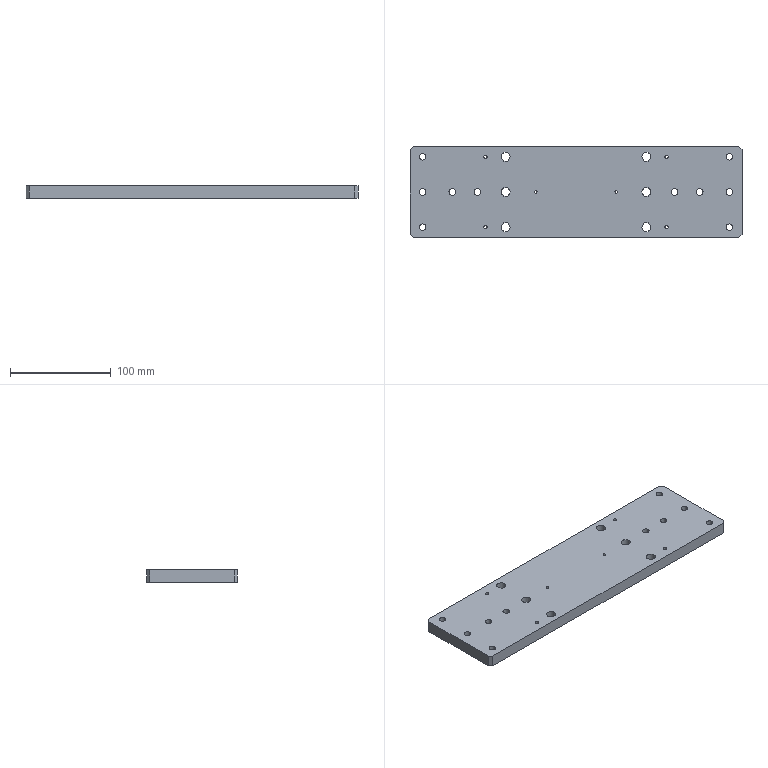Part | 1 solid | 52 faces | box 330 x 90 x 12 mm | volume 343077 mm3 | cylinder 32 | plane 20 | commonest cylinder face diameters 6.6 x10 11 x10 9 x6 3.3 x4 2.5 x2
STEP:
#1=CARTESIAN_POINT('',(147.,35.,0.4));
#2=VERTEX_POINT('',#1);
#3=CARTESIAN_POINT('',(152.5,35.,0.4));
#4=DIRECTION('',(0.,0.,-1.));
#5=DIRECTION('',(-1.,0.,0.));
#6=AXIS2_PLACEMENT_3D('',#3,#4,#5);
#7=CIRCLE('',#6,5.5);
#8=EDGE_CURVE('',#2,#2,#7,.T.);
#9=ORIENTED_EDGE('',*,*,#8,.T.);
#10=EDGE_LOOP('',(#9));
#11=FACE_BOUND('',#10,.T.);
#12=CARTESIAN_POINT('',(149.2,35.,0.4));
#13=VERTEX_POINT('',#12);
#14=CARTESIAN_POINT('',(152.5,35.,0.4));
#15=DIRECTION('',(0.,0.,-1.));
#16=DIRECTION('',(-1.,0.,0.));
#17=AXIS2_PLACEMENT_3D('',#14,#15,#16);
#18=CIRCLE('',#17,3.3);
#19=EDGE_CURVE('',#13,#13,#18,.T.);
#20=ORIENTED_EDGE('',*,*,#19,.F.);
#21=EDGE_LOOP('',(#20));
#22=FACE_BOUND('',#21,.T.);
#23=CARTESIAN_POINT('',(155.8,35.,0.4));
#24=DIRECTION('',(0.,0.,1.));
#25=DIRECTION('',(1.,0.,0.));
#26=AXIS2_PLACEMENT_3D('',#23,#24,#25);
#27=PLANE('',#26);
#28=ADVANCED_FACE('',(#11,#22),#27,.F.);
#29=CARTESIAN_POINT('',(158.,0.,0.4));
#30=VERTEX_POINT('',#29);
#31=CARTESIAN_POINT('',(152.5,0.,0.4));
#32=DIRECTION('',(0.,0.,-1.));
#33=DIRECTION('',(1.,0.,0.));
#34=AXIS2_PLACEMENT_3D('',#31,#32,#33);
#35=CIRCLE('',#34,5.5);
#36=EDGE_CURVE('',#30,#30,#35,.T.);
#37=ORIENTED_EDGE('',*,*,#36,.T.);
#38=EDGE_LOOP('',(#37));
#39=FACE_BOUND('',#38,.T.);
#40=CARTESIAN_POINT('',(155.8,0.,0.4));
#41=VERTEX_POINT('',#40);
#42=CARTESIAN_POINT('',(152.5,0.,0.4));
#43=DIRECTION('',(0.,0.,-1.));
#44=DIRECTION('',(1.,0.,0.));
#45=AXIS2_PLACEMENT_3D('',#42,#43,#44);
#46=CIRCLE('',#45,3.3);
#47=EDGE_CURVE('',#41,#41,#46,.T.);
#48=ORIENTED_EDGE('',*,*,#47,.F.);
#49=EDGE_LOOP('',(#48));
#50=FACE_BOUND('',#49,.T.);
#51=CARTESIAN_POINT('',(155.8,35.,0.4));
#52=DIRECTION('',(0.,0.,1.));
#53=DIRECTION('',(1.,0.,0.));
#54=AXIS2_PLACEMENT_3D('',#51,#52,#53);
#55=PLANE('',#54);
#56=ADVANCED_FACE('',(#39,#50),#55,.F.);
#57=CARTESIAN_POINT('',(128.5,0.,0.4));
#58=VERTEX_POINT('',#57);
#59=CARTESIAN_POINT('',(123.,0.,0.4));
#60=DIRECTION('',(0.,0.,-1.));
#61=DIRECTION('',(1.,0.,0.));
#62=AXIS2_PLACEMENT_3D('',#59,#60,#61);
#63=CIRCLE('',#62,5.5);
#64=EDGE_CURVE('',#58,#58,#63,.T.);
#65=ORIENTED_EDGE('',*,*,#64,.T.);
#66=EDGE_LOOP('',(#65));
#67=FACE_BOUND('',#66,.T.);
#68=CARTESIAN_POINT('',(126.3,0.,0.4));
#69=VERTEX_POINT('',#68);
#70=CARTESIAN_POINT('',(123.,0.,0.4));
#71=DIRECTION('',(0.,0.,-1.));
#72=DIRECTION('',(1.,0.,0.));
#73=AXIS2_PLACEMENT_3D('',#70,#71,#72);
#74=CIRCLE('',#73,3.3);
#75=EDGE_CURVE('',#69,#69,#74,.T.);
#76=ORIENTED_EDGE('',*,*,#75,.F.);
#77=EDGE_LOOP('',(#76));
#78=FACE_BOUND('',#77,.T.);
#79=CARTESIAN_POINT('',(155.8,35.,0.4));
#80=DIRECTION('',(0.,0.,1.));
#81=DIRECTION('',(1.,0.,0.));
#82=AXIS2_PLACEMENT_3D('',#79,#80,#81);
#83=PLANE('',#82);
#84=ADVANCED_FACE('',(#67,#78),#83,.F.);
#85=CARTESIAN_POINT('',(103.5,0.,0.4));
#86=VERTEX_POINT('',#85);
#87=CARTESIAN_POINT('',(98.,0.,0.4));
#88=DIRECTION('',(0.,0.,-1.));
#89=DIRECTION('',(1.,0.,0.));
#90=AXIS2_PLACEMENT_3D('',#87,#88,#89);
#91=CIRCLE('',#90,5.5);
#92=EDGE_CURVE('',#86,#86,#91,.T.);
#93=ORIENTED_EDGE('',*,*,#92,.T.);
#94=EDGE_LOOP('',(#93));
#95=FACE_BOUND('',#94,.T.);
#96=CARTESIAN_POINT('',(101.3,0.,0.4));
#97=VERTEX_POINT('',#96);
#98=CARTESIAN_POINT('',(98.,0.,0.4));
#99=DIRECTION('',(0.,0.,-1.));
#100=DIRECTION('',(1.,0.,0.));
#101=AXIS2_PLACEMENT_3D('',#98,#99,#100);
#102=CIRCLE('',#101,3.3);
#103=EDGE_CURVE('',#97,#97,#102,.T.);
#104=ORIENTED_EDGE('',*,*,#103,.F.);
#105=EDGE_LOOP('',(#104));
#106=FACE_BOUND('',#105,.T.);
#107=CARTESIAN_POINT('',(155.8,35.,0.4));
#108=DIRECTION('',(0.,0.,1.));
#109=DIRECTION('',(1.,0.,0.));
#110=AXIS2_PLACEMENT_3D('',#107,#108,#109);
#111=PLANE('',#110);
#112=ADVANCED_FACE('',(#95,#106),#111,.F.);
#113=CARTESIAN_POINT('',(158.,-35.,0.4));
#114=VERTEX_POINT('',#113);
#115=CARTESIAN_POINT('',(152.5,-35.,0.4));
#116=DIRECTION('',(0.,0.,-1.));
#117=DIRECTION('',(1.,0.,0.));
#118=AXIS2_PLACEMENT_3D('',#115,#116,#117);
#119=CIRCLE('',#118,5.5);
#120=EDGE_CURVE('',#114,#114,#119,.T.);
#121=ORIENTED_EDGE('',*,*,#120,.T.);
#122=EDGE_LOOP('',(#121));
#123=FACE_BOUND('',#122,.T.);
#124=CARTESIAN_POINT('',(155.8,-35.,0.4));
#125=VERTEX_POINT('',#124);
#126=CARTESIAN_POINT('',(152.5,-35.,0.4));
#127=DIRECTION('',(0.,0.,-1.));
#128=DIRECTION('',(1.,0.,0.));
#129=AXIS2_PLACEMENT_3D('',#126,#127,#128);
#130=CIRCLE('',#129,3.3);
#131=EDGE_CURVE('',#125,#125,#130,.T.);
#132=ORIENTED_EDGE('',*,*,#131,.F.);
#133=EDGE_LOOP('',(#132));
#134=FACE_BOUND('',#133,.T.);
#135=CARTESIAN_POINT('',(155.8,35.,0.4));
#136=DIRECTION('',(0.,0.,1.));
#137=DIRECTION('',(1.,0.,0.));
#138=AXIS2_PLACEMENT_3D('',#135,#136,#137);
#139=PLANE('',#138);
#140=ADVANCED_FACE('',(#123,#134),#139,.F.);
#141=CARTESIAN_POINT('',(-147.,-35.,0.4));
#142=VERTEX_POINT('',#141);
#143=CARTESIAN_POINT('',(-152.5,-35.,0.4));
#144=DIRECTION('',(0.,0.,-1.));
#145=DIRECTION('',(1.,0.,0.));
#146=AXIS2_PLACEMENT_3D('',#143,#144,#145);
#147=CIRCLE('',#146,5.5);
#148=EDGE_CURVE('',#142,#142,#147,.T.);
#149=ORIENTED_EDGE('',*,*,#148,.T.);
#150=EDGE_LOOP('',(#149));
#151=FACE_BOUND('',#150,.T.);
#152=CARTESIAN_POINT('',(-149.2,-35.,0.4));
#153=VERTEX_POINT('',#152);
#154=CARTESIAN_POINT('',(-152.5,-35.,0.4));
#155=DIRECTION('',(0.,0.,-1.));
#156=DIRECTION('',(1.,0.,0.));
#157=AXIS2_PLACEMENT_3D('',#154,#155,#156);
#158=CIRCLE('',#157,3.3);
#159=EDGE_CURVE('',#153,#153,#158,.T.);
#160=ORIENTED_EDGE('',*,*,#159,.F.);
#161=EDGE_LOOP('',(#160));
#162=FACE_BOUND('',#161,.T.);
#163=CARTESIAN_POINT('',(155.8,35.,0.4));
#164=DIRECTION('',(0.,0.,1.));
#165=DIRECTION('',(1.,0.,0.));
#166=AXIS2_PLACEMENT_3D('',#163,#164,#165);
#167=PLANE('',#166);
#168=ADVANCED_FACE('',(#151,#162),#167,.F.);
#169=CARTESIAN_POINT('',(-92.5,0.,0.4));
#170=VERTEX_POINT('',#169);
#171=CARTESIAN_POINT('',(-98.,0.,0.4));
#172=DIRECTION('',(0.,0.,-1.));
#173=DIRECTION('',(1.,0.,0.));
#174=AXIS2_PLACEMENT_3D('',#171,#172,#173);
#175=CIRCLE('',#174,5.5);
#176=EDGE_CURVE('',#170,#170,#175,.T.);
#177=ORIENTED_EDGE('',*,*,#176,.T.);
#178=EDGE_LOOP('',(#177));
#179=FACE_BOUND('',#178,.T.);
#180=CARTESIAN_POINT('',(-94.7,0.,0.4));
#181=VERTEX_POINT('',#180);
#182=CARTESIAN_POINT('',(-98.,0.,0.4));
#183=DIRECTION('',(0.,0.,-1.));
#184=DIRECTION('',(1.,0.,0.));
#185=AXIS2_PLACEMENT_3D('',#182,#183,#184);
#186=CIRCLE('',#185,3.3);
#187=EDGE_CURVE('',#181,#181,#186,.T.);
#188=ORIENTED_EDGE('',*,*,#187,.F.);
#189=EDGE_LOOP('',(#188));
#190=FACE_BOUND('',#189,.T.);
#191=CARTESIAN_POINT('',(155.8,35.,0.4));
#192=DIRECTION('',(0.,0.,1.));
#193=DIRECTION('',(1.,0.,0.));
#194=AXIS2_PLACEMENT_3D('',#191,#192,#193);
#195=PLANE('',#194);
#196=ADVANCED_FACE('',(#179,#190),#195,.F.);
#197=CARTESIAN_POINT('',(-117.5,0.,0.4));
#198=VERTEX_POINT('',#197);
#199=CARTESIAN_POINT('',(-123.,0.,0.4));
#200=DIRECTION('',(0.,0.,-1.));
#201=DIRECTION('',(1.,0.,0.));
#202=AXIS2_PLACEMENT_3D('',#199,#200,#201);
#203=CIRCLE('',#202,5.5);
#204=EDGE_CURVE('',#198,#198,#203,.T.);
#205=ORIENTED_EDGE('',*,*,#204,.T.);
#206=EDGE_LOOP('',(#205));
#207=FACE_BOUND('',#206,.T.);
#208=CARTESIAN_POINT('',(-119.7,0.,0.4));
#209=VERTEX_POINT('',#208);
#210=CARTESIAN_POINT('',(-123.,0.,0.4));
#211=DIRECTION('',(0.,0.,-1.));
#212=DIRECTION('',(1.,0.,0.));
#213=AXIS2_PLACEMENT_3D('',#210,#211,#212);
#214=CIRCLE('',#213,3.3);
#215=EDGE_CURVE('',#209,#209,#214,.T.);
#216=ORIENTED_EDGE('',*,*,#215,.F.);
#217=EDGE_LOOP('',(#216));
#218=FACE_BOUND('',#217,.T.);
#219=CARTESIAN_POINT('',(155.8,35.,0.4));
#220=DIRECTION('',(0.,0.,1.));
#221=DIRECTION('',(1.,0.,0.));
#222=AXIS2_PLACEMENT_3D('',#219,#220,#221);
#223=PLANE('',#222);
#224=ADVANCED_FACE('',(#207,#218),#223,.F.);
#225=CARTESIAN_POINT('',(-147.,0.,0.4));
#226=VERTEX_POINT('',#225);
#227=CARTESIAN_POINT('',(-152.5,0.,0.4));
#228=DIRECTION('',(0.,0.,-1.));
#229=DIRECTION('',(1.,0.,0.));
#230=AXIS2_PLACEMENT_3D('',#227,#228,#229);
#231=CIRCLE('',#230,5.5);
#232=EDGE_CURVE('',#226,#226,#231,.T.);
#233=ORIENTED_EDGE('',*,*,#232,.T.);
#234=EDGE_LOOP('',(#233));
#235=FACE_BOUND('',#234,.T.);
#236=CARTESIAN_POINT('',(-149.2,0.,0.4));
#237=VERTEX_POINT('',#236);
#238=CARTESIAN_POINT('',(-152.5,0.,0.4));
#239=DIRECTION('',(0.,0.,-1.));
#240=DIRECTION('',(1.,0.,0.));
#241=AXIS2_PLACEMENT_3D('',#238,#239,#240);
#242=CIRCLE('',#241,3.3);
#243=EDGE_CURVE('',#237,#237,#242,.T.);
#244=ORIENTED_EDGE('',*,*,#243,.F.);
#245=EDGE_LOOP('',(#244));
#246=FACE_BOUND('',#245,.T.);
#247=CARTESIAN_POINT('',(155.8,35.,0.4));
#248=DIRECTION('',(0.,0.,1.));
#249=DIRECTION('',(1.,0.,0.));
#250=AXIS2_PLACEMENT_3D('',#247,#248,#249);
#251=PLANE('',#250);
#252=ADVANCED_FACE('',(#235,#246),#251,.F.);
#253=CARTESIAN_POINT('',(-147.,35.,0.4));
#254=VERTEX_POINT('',#253);
#255=CARTESIAN_POINT('',(-152.5,35.,0.4));
#256=DIRECTION('',(0.,0.,-1.));
#257=DIRECTION('',(1.,0.,0.));
#258=AXIS2_PLACEMENT_3D('',#255,#256,#257);
#259=CIRCLE('',#258,5.5);
#260=EDGE_CURVE('',#254,#254,#259,.T.);
#261=ORIENTED_EDGE('',*,*,#260,.T.);
#262=EDGE_LOOP('',(#261));
#263=FACE_BOUND('',#262,.T.);
#264=CARTESIAN_POINT('',(-149.2,35.,0.4));
#265=VERTEX_POINT('',#264);
#266=CARTESIAN_POINT('',(-152.5,35.,0.4));
#267=DIRECTION('',(0.,0.,-1.));
#268=DIRECTION('',(1.,0.,0.));
#269=AXIS2_PLACEMENT_3D('',#266,#267,#268);
#270=CIRCLE('',#269,3.3);
#271=EDGE_CURVE('',#265,#265,#270,.T.);
#272=ORIENTED_EDGE('',*,*,#271,.F.);
#273=EDGE_LOOP('',(#272));
#274=FACE_BOUND('',#273,.T.);
#275=CARTESIAN_POINT('',(155.8,35.,0.4));
#276=DIRECTION('',(0.,0.,1.));
#277=DIRECTION('',(1.,0.,0.));
#278=AXIS2_PLACEMENT_3D('',#275,#276,#277);
#279=PLANE('',#278);
#280=ADVANCED_FACE('',(#263,#274),#279,.F.);
#281=CARTESIAN_POINT('',(-165.,-42.,6.));
#282=VERTEX_POINT('',#281);
#283=CARTESIAN_POINT('',(-162.,-45.,6.));
#284=VERTEX_POINT('',#283);
#285=CARTESIAN_POINT('',(-103.5,-103.5,6.));
#286=DIRECTION('',(0.7071,-0.7071,0.));
#287=VECTOR('',#286,1000.);
#288=LINE('',#285,#287);
#289=EDGE_CURVE('',#282,#284,#288,.T.);
#290=ORIENTED_EDGE('',*,*,#289,.F.);
#291=CARTESIAN_POINT('',(-165.,-42.,-6.));
#292=VERTEX_POINT('',#291);
#293=CARTESIAN_POINT('',(-165.,-42.,6.));
#294=DIRECTION('',(0.,0.,1.));
#295=VECTOR('',#294,1000.);
#296=LINE('',#293,#295);
#297=EDGE_CURVE('',#292,#282,#296,.T.);
#298=ORIENTED_EDGE('',*,*,#297,.F.);
#299=CARTESIAN_POINT('',(-162.,-45.,-6.));
#300=VERTEX_POINT('',#299);
#301=CARTESIAN_POINT('',(-162.,-45.,-6.));
#302=DIRECTION('',(-0.7071,0.7071,0.));
#303=VECTOR('',#302,1000.);
#304=LINE('',#301,#303);
#305=EDGE_CURVE('',#300,#292,#304,.T.);
#306=ORIENTED_EDGE('',*,*,#305,.F.);
#307=CARTESIAN_POINT('',(-162.,-45.,6.));
#308=DIRECTION('',(0.,0.,-1.));
#309=VECTOR('',#308,1000.);
#310=LINE('',#307,#309);
#311=EDGE_CURVE('',#284,#300,#310,.T.);
#312=ORIENTED_EDGE('',*,*,#311,.F.);
#313=EDGE_LOOP('',(#290,#298,#306,#312));
#314=FACE_BOUND('',#313,.T.);
#315=CARTESIAN_POINT('',(-162.,-45.,6.));
#316=DIRECTION('',(0.7071,0.7071,0.));
#317=DIRECTION('',(0.,0.,-1.));
#318=AXIS2_PLACEMENT_3D('',#315,#316,#317);
#319=PLANE('',#318);
#320=ADVANCED_FACE('',(#314),#319,.F.);
#321=CARTESIAN_POINT('',(-162.,45.,6.));
#322=VERTEX_POINT('',#321);
#323=CARTESIAN_POINT('',(-165.,42.,6.));
#324=VERTEX_POINT('',#323);
#325=CARTESIAN_POINT('',(-103.5,103.5,6.));
#326=DIRECTION('',(-0.7071,-0.7071,0.));
#327=VECTOR('',#326,1000.);
#328=LINE('',#325,#327);
#329=EDGE_CURVE('',#322,#324,#328,.T.);
#330=ORIENTED_EDGE('',*,*,#329,.F.);
#331=CARTESIAN_POINT('',(-162.,45.,-6.));
#332=VERTEX_POINT('',#331);
#333=CARTESIAN_POINT('',(-162.,45.,6.));
#334=DIRECTION('',(0.,0.,1.));
#335=VECTOR('',#334,1000.);
#336=LINE('',#333,#335);
#337=EDGE_CURVE('',#332,#322,#336,.T.);
#338=ORIENTED_EDGE('',*,*,#337,.F.);
#339=CARTESIAN_POINT('',(-165.,42.,-6.));
#340=VERTEX_POINT('',#339);
#341=CARTESIAN_POINT('',(-165.,42.,-6.));
#342=DIRECTION('',(0.7071,0.7071,0.));
#343=VECTOR('',#342,1000.);
#344=LINE('',#341,#343);
#345=EDGE_CURVE('',#340,#332,#344,.T.);
#346=ORIENTED_EDGE('',*,*,#345,.F.);
#347=CARTESIAN_POINT('',(-165.,42.,6.));
#348=DIRECTION('',(0.,0.,-1.));
#349=VECTOR('',#348,1000.);
#350=LINE('',#347,#349);
#351=EDGE_CURVE('',#324,#340,#350,.T.);
#352=ORIENTED_EDGE('',*,*,#351,.F.);
#353=EDGE_LOOP('',(#330,#338,#346,#352));
#354=FACE_BOUND('',#353,.T.);
#355=CARTESIAN_POINT('',(-165.,42.,6.));
#356=DIRECTION('',(0.7071,-0.7071,0.));
#357=DIRECTION('',(0.,0.,-1.));
#358=AXIS2_PLACEMENT_3D('',#355,#356,#357);
#359=PLANE('',#358);
#360=ADVANCED_FACE('',(#354),#359,.F.);
#361=CARTESIAN_POINT('',(165.,42.,6.));
#362=VERTEX_POINT('',#361);
#363=CARTESIAN_POINT('',(162.,45.,6.));
#364=VERTEX_POINT('',#363);
#365=CARTESIAN_POINT('',(103.5,103.5,6.));
#366=DIRECTION('',(-0.7071,0.7071,0.));
#367=VECTOR('',#366,1000.);
#368=LINE('',#365,#367);
#369=EDGE_CURVE('',#362,#364,#368,.T.);
#370=ORIENTED_EDGE('',*,*,#369,.F.);
#371=CARTESIAN_POINT('',(165.,42.,-6.));
#372=VERTEX_POINT('',#371);
#373=CARTESIAN_POINT('',(165.,42.,6.));
#374=DIRECTION('',(0.,0.,1.));
#375=VECTOR('',#374,1000.);
#376=LINE('',#373,#375);
#377=EDGE_CURVE('',#372,#362,#376,.T.);
#378=ORIENTED_EDGE('',*,*,#377,.F.);
#379=CARTESIAN_POINT('',(162.,45.,-6.));
#380=VERTEX_POINT('',#379);
#381=CARTESIAN_POINT('',(162.,45.,-6.));
#382=DIRECTION('',(0.7071,-0.7071,0.));
#383=VECTOR('',#382,1000.);
#384=LINE('',#381,#383);
#385=EDGE_CURVE('',#380,#372,#384,.T.);
#386=ORIENTED_EDGE('',*,*,#385,.F.);
#387=CARTESIAN_POINT('',(162.,45.,6.));
#388=DIRECTION('',(0.,0.,-1.));
#389=VECTOR('',#388,1000.);
#390=LINE('',#387,#389);
#391=EDGE_CURVE('',#364,#380,#390,.T.);
#392=ORIENTED_EDGE('',*,*,#391,.F.);
#393=EDGE_LOOP('',(#370,#378,#386,#392));
#394=FACE_BOUND('',#393,.T.);
#395=CARTESIAN_POINT('',(162.,45.,6.));
#396=DIRECTION('',(-0.7071,-0.7071,0.));
#397=DIRECTION('',(0.,0.,-1.));
#398=AXIS2_PLACEMENT_3D('',#395,#396,#397);
#399=PLANE('',#398);
#400=ADVANCED_FACE('',(#394),#399,.F.);
#401=CARTESIAN_POINT('',(162.,-45.,6.));
#402=VERTEX_POINT('',#401);
#403=CARTESIAN_POINT('',(165.,-42.,6.));
#404=VERTEX_POINT('',#403);
#405=CARTESIAN_POINT('',(103.5,-103.5,6.));
#406=DIRECTION('',(0.7071,0.7071,0.));
#407=VECTOR('',#406,1000.);
#408=LINE('',#405,#407);
#409=EDGE_CURVE('',#402,#404,#408,.T.);
#410=ORIENTED_EDGE('',*,*,#409,.F.);
#411=CARTESIAN_POINT('',(162.,-45.,-6.));
#412=VERTEX_POINT('',#411);
#413=CARTESIAN_POINT('',(162.,-45.,6.));
#414=DIRECTION('',(0.,0.,1.));
#415=VECTOR('',#414,1000.);
#416=LINE('',#413,#415);
#417=EDGE_CURVE('',#412,#402,#416,.T.);
#418=ORIENTED_EDGE('',*,*,#417,.F.);
#419=CARTESIAN_POINT('',(165.,-42.,-6.));
#420=VERTEX_POINT('',#419);
#421=CARTESIAN_POINT('',(165.,-42.,-6.));
#422=DIRECTION('',(-0.7071,-0.7071,0.));
#423=VECTOR('',#422,1000.);
#424=LINE('',#421,#423);
#425=EDGE_CURVE('',#420,#412,#424,.T.);
#426=ORIENTED_EDGE('',*,*,#425,.F.);
#427=CARTESIAN_POINT('',(165.,-42.,6.));
#428=DIRECTION('',(0.,0.,-1.));
#429=VECTOR('',#428,1000.);
#430=LINE('',#427,#429);
#431=EDGE_CURVE('',#404,#420,#430,.T.);
#432=ORIENTED_EDGE('',*,*,#431,.F.);
#433=EDGE_LOOP('',(#410,#418,#426,#432));
#434=FACE_BOUND('',#433,.T.);
#435=CARTESIAN_POINT('',(165.,-42.,6.));
#436=DIRECTION('',(-0.7071,0.7071,0.));
#437=DIRECTION('',(0.,0.,-1.));
#438=AXIS2_PLACEMENT_3D('',#435,#436,#437);
#439=PLANE('',#438);
#440=ADVANCED_FACE('',(#434),#439,.F.);
#441=CARTESIAN_POINT('',(165.,45.,-6.));
#442=DIRECTION('',(0.,1.,0.));
#443=VECTOR('',#442,1000.);
#444=LINE('',#441,#443);
#445=EDGE_CURVE('',#420,#372,#444,.T.);
#446=ORIENTED_EDGE('',*,*,#445,.F.);
#447=ORIENTED_EDGE('',*,*,#425,.T.);
#448=CARTESIAN_POINT('',(-165.,-45.,-6.));
#449=DIRECTION('',(1.,0.,0.));
#450=VECTOR('',#449,1000.);
#451=LINE('',#448,#450);
#452=EDGE_CURVE('',#300,#412,#451,.T.);
#453=ORIENTED_EDGE('',*,*,#452,.F.);
#454=ORIENTED_EDGE('',*,*,#305,.T.);
#455=CARTESIAN_POINT('',(-165.,45.,-6.));
#456=DIRECTION('',(0.,-1.,0.));
#457=VECTOR('',#456,1000.);
#458=LINE('',#455,#457);
#459=EDGE_CURVE('',#340,#292,#458,.T.);
#460=ORIENTED_EDGE('',*,*,#459,.F.);
#461=ORIENTED_EDGE('',*,*,#345,.T.);
#462=CARTESIAN_POINT('',(-165.,45.,-6.));
#463=DIRECTION('',(-1.,0.,0.));
#464=VECTOR('',#463,1000.);
#465=LINE('',#462,#464);
#466=EDGE_CURVE('',#380,#332,#465,.T.);
#467=ORIENTED_EDGE('',*,*,#466,.F.);
#468=ORIENTED_EDGE('',*,*,#385,.T.);
#469=EDGE_LOOP('',(#446,#447,#453,#454,#460,#461,#467,#468));
#470=FACE_BOUND('',#469,.T.);
#471=CARTESIAN_POINT('',(-65.5,-35.,-6.));
#472=VERTEX_POINT('',#471);
#473=CARTESIAN_POINT('',(-70.,-35.,-6.));
#474=DIRECTION('',(0.,0.,1.));
#475=DIRECTION('',(1.,0.,0.));
#476=AXIS2_PLACEMENT_3D('',#473,#474,#475);
#477=CIRCLE('',#476,4.5);
#478=EDGE_CURVE('',#472,#472,#477,.T.);
#479=ORIENTED_EDGE('',*,*,#478,.T.);
#480=EDGE_LOOP('',(#479));
#481=FACE_BOUND('',#480,.T.);
#482=CARTESIAN_POINT('',(-65.5,0.,-6.));
#483=VERTEX_POINT('',#482);
#484=CARTESIAN_POINT('',(-70.,0.,-6.));
#485=DIRECTION('',(0.,0.,1.));
#486=DIRECTION('',(1.,0.,0.));
#487=AXIS2_PLACEMENT_3D('',#484,#485,#486);
#488=CIRCLE('',#487,4.5);
#489=EDGE_CURVE('',#483,#483,#488,.T.);
#490=ORIENTED_EDGE('',*,*,#489,.T.);
#491=EDGE_LOOP('',(#490));
#492=FACE_BOUND('',#491,.T.);
#493=CARTESIAN_POINT('',(-65.5,35.,-6.));
#494=VERTEX_POINT('',#493);
#495=CARTESIAN_POINT('',(-70.,35.,-6.));
#496=DIRECTION('',(0.,0.,1.));
#497=DIRECTION('',(1.,0.,0.));
#498=AXIS2_PLACEMENT_3D('',#495,#496,#497);
#499=CIRCLE('',#498,4.5);
#500=EDGE_CURVE('',#494,#494,#499,.T.);
#501=ORIENTED_EDGE('',*,*,#500,.T.);
#502=EDGE_LOOP('',(#501));
#503=FACE_BOUND('',#502,.T.);
#504=CARTESIAN_POINT('',(74.5,35.,-6.));
#505=VERTEX_POINT('',#504);
#506=CARTESIAN_POINT('',(70.,35.,-6.));
#507=DIRECTION('',(0.,0.,1.));
#508=DIRECTION('',(1.,0.,0.));
#509=AXIS2_PLACEMENT_3D('',#506,#507,#508);
#510=CIRCLE('',#509,4.5);
#511=EDGE_CURVE('',#505,#505,#510,.T.);
#512=ORIENTED_EDGE('',*,*,#511,.T.);
#513=EDGE_LOOP('',(#512));
#514=FACE_BOUND('',#513,.T.);
#515=CARTESIAN_POINT('',(74.5,0.,-6.));
#516=VERTEX_POINT('',#515);
#517=CARTESIAN_POINT('',(70.,0.,-6.));
#518=DIRECTION('',(0.,0.,1.));
#519=DIRECTION('',(1.,0.,0.));
#520=AXIS2_PLACEMENT_3D('',#517,#518,#519);
#521=CIRCLE('',#520,4.5);
#522=EDGE_CURVE('',#516,#516,#521,.T.);
#523=ORIENTED_EDGE('',*,*,#522,.T.);
#524=EDGE_LOOP('',(#523));
#525=FACE_BOUND('',#524,.T.);
#526=CARTESIAN_POINT('',(74.5,-35.,-6.));
#527=VERTEX_POINT('',#526);
#528=CARTESIAN_POINT('',(70.,-35.,-6.));
#529=DIRECTION('',(0.,0.,1.));
#530=DIRECTION('',(1.,0.,0.));
#531=AXIS2_PLACEMENT_3D('',#528,#529,#530);
#532=CIRCLE('',#531,4.5);
#533=EDGE_CURVE('',#527,#527,#532,.T.);
#534=ORIENTED_EDGE('',*,*,#533,.T.);
#535=EDGE_LOOP('',(#534));
#536=FACE_BOUND('',#535,.T.);
#537=CARTESIAN_POINT('',(-158.,35.,-6.));
#538=VERTEX_POINT('',#537);
#539=CARTESIAN_POINT('',(-152.5,35.,-6.));
#540=DIRECTION('',(0.,0.,-1.));
#541=DIRECTION('',(-1.,0.,0.));
#542=AXIS2_PLACEMENT_3D('',#539,#540,#541);
#543=CIRCLE('',#542,5.5);
#544=EDGE_CURVE('',#538,#538,#543,.T.);
#545=ORIENTED_EDGE('',*,*,#544,.F.);
#546=EDGE_LOOP('',(#545));
#547=FACE_BOUND('',#546,.T.);
#548=CARTESIAN_POINT('',(-158.,0.,-6.));
#549=VERTEX_POINT('',#548);
#550=CARTESIAN_POINT('',(-152.5,0.,-6.));
#551=DIRECTION('',(0.,0.,-1.));
#552=DIRECTION('',(-1.,0.,0.));
#553=AXIS2_PLACEMENT_3D('',#550,#551,#552);
#554=CIRCLE('',#553,5.5);
#555=EDGE_CURVE('',#549,#549,#554,.T.);
#556=ORIENTED_EDGE('',*,*,#555,.F.);
#557=EDGE_LOOP('',(#556));
#558=FACE_BOUND('',#557,.T.);
#559=CARTESIAN_POINT('',(-128.5,0.,-6.));
#560=VERTEX_POINT('',#559);
#561=CARTESIAN_POINT('',(-123.,0.,-6.));
#562=DIRECTION('',(0.,0.,-1.));
#563=DIRECTION('',(-1.,0.,0.));
#564=AXIS2_PLACEMENT_3D('',#561,#562,#563);
#565=CIRCLE('',#564,5.5);
#566=EDGE_CURVE('',#560,#560,#565,.T.);
#567=ORIENTED_EDGE('',*,*,#566,.F.);
#568=EDGE_LOOP('',(#567));
#569=FACE_BOUND('',#568,.T.);
#570=CARTESIAN_POINT('',(-103.5,0.,-6.));
#571=VERTEX_POINT('',#570);
#572=CARTESIAN_POINT('',(-98.,0.,-6.));
#573=DIRECTION('',(0.,0.,-1.));
#574=DIRECTION('',(-1.,0.,0.));
#575=AXIS2_PLACEMENT_3D('',#572,#573,#574);
#576=CIRCLE('',#575,5.5);
#577=EDGE_CURVE('',#571,#571,#576,.T.);
#578=ORIENTED_EDGE('',*,*,#577,.F.);
#579=EDGE_LOOP('',(#578));
#580=FACE_BOUND('',#579,.T.);
#581=CARTESIAN_POINT('',(-158.,-35.,-6.));
#582=VERTEX_POINT('',#581);
#583=CARTESIAN_POINT('',(-152.5,-35.,-6.));
#584=DIRECTION('',(0.,0.,-1.));
#585=DIRECTION('',(-1.,0.,0.));
#586=AXIS2_PLACEMENT_3D('',#583,#584,#585);
#587=CIRCLE('',#586,5.5);
#588=EDGE_CURVE('',#582,#582,#587,.T.);
#589=ORIENTED_EDGE('',*,*,#588,.F.);
#590=EDGE_LOOP('',(#589));
#591=FACE_BOUND('',#590,.T.);
#592=CARTESIAN_POINT('',(147.,-35.,-6.));
#593=VERTEX_POINT('',#592);
#594=CARTESIAN_POINT('',(152.5,-35.,-6.));
#595=DIRECTION('',(0.,0.,-1.));
#596=DIRECTION('',(-1.,0.,0.));
#597=AXIS2_PLACEMENT_3D('',#594,#595,#596);
#598=CIRCLE('',#597,5.5);
#599=EDGE_CURVE('',#593,#593,#598,.T.);
#600=ORIENTED_EDGE('',*,*,#599,.F.);
#601=EDGE_LOOP('',(#600));
#602=FACE_BOUND('',#601,.T.);
#603=CARTESIAN_POINT('',(92.5,0.,-6.));
#604=VERTEX_POINT('',#603);
#605=CARTESIAN_POINT('',(98.,0.,-6.));
#606=DIRECTION('',(0.,0.,-1.));
#607=DIRECTION('',(-1.,0.,0.));
#608=AXIS2_PLACEMENT_3D('',#605,#606,#607);
#609=CIRCLE('',#608,5.5);
#610=EDGE_CURVE('',#604,#604,#609,.T.);
#611=ORIENTED_EDGE('',*,*,#610,.F.);
#612=EDGE_LOOP('',(#611));
#613=FACE_BOUND('',#612,.T.);
#614=CARTESIAN_POINT('',(117.5,0.,-6.));
#615=VERTEX_POINT('',#614);
#616=CARTESIAN_POINT('',(123.,0.,-6.));
#617=DIRECTION('',(0.,0.,-1.));
#618=DIRECTION('',(-1.,0.,0.));
#619=AXIS2_PLACEMENT_3D('',#616,#617,#618);
#620=CIRCLE('',#619,5.5);
#621=EDGE_CURVE('',#615,#615,#620,.T.);
#622=ORIENTED_EDGE('',*,*,#621,.F.);
#623=EDGE_LOOP('',(#622));
#624=FACE_BOUND('',#623,.T.);
#625=CARTESIAN_POINT('',(147.,0.,-6.));
#626=VERTEX_POINT('',#625);
#627=CARTESIAN_POINT('',(152.5,0.,-6.));
#628=DIRECTION('',(0.,0.,-1.));
#629=DIRECTION('',(-1.,0.,0.));
#630=AXIS2_PLACEMENT_3D('',#627,#628,#629);
#631=CIRCLE('',#630,5.5);
#632=EDGE_CURVE('',#626,#626,#631,.T.);
#633=ORIENTED_EDGE('',*,*,#632,.F.);
#634=EDGE_LOOP('',(#633));
#635=FACE_BOUND('',#634,.T.);
#636=CARTESIAN_POINT('',(147.,35.,-6.));
#637=VERTEX_POINT('',#636);
#638=CARTESIAN_POINT('',(152.5,35.,-6.));
#639=DIRECTION('',(0.,0.,-1.));
#640=DIRECTION('',(-1.,0.,0.));
#641=AXIS2_PLACEMENT_3D('',#638,#639,#640);
#642=CIRCLE('',#641,5.5);
#643=EDGE_CURVE('',#637,#637,#642,.T.);
#644=ORIENTED_EDGE('',*,*,#643,.F.);
#645=EDGE_LOOP('',(#644));
#646=FACE_BOUND('',#645,.T.);
#647=CARTESIAN_POINT('',(41.25,0.,-6.));
#648=VERTEX_POINT('',#647);
#649=CARTESIAN_POINT('',(40.,0.,-6.));
#650=DIRECTION('',(0.,0.,1.));
#651=DIRECTION('',(1.,0.,0.));
#652=AXIS2_PLACEMENT_3D('',#649,#650,#651);
#653=CIRCLE('',#652,1.25);
#654=EDGE_CURVE('',#648,#648,#653,.T.);
#655=ORIENTED_EDGE('',*,*,#654,.T.);
#656=EDGE_LOOP('',(#655));
#657=FACE_BOUND('',#656,.T.);
#658=CARTESIAN_POINT('',(-38.75,0.,-6.));
#659=VERTEX_POINT('',#658);
#660=CARTESIAN_POINT('',(-40.,0.,-6.));
#661=DIRECTION('',(0.,0.,1.));
#662=DIRECTION('',(1.,0.,0.));
#663=AXIS2_PLACEMENT_3D('',#660,#661,#662);
#664=CIRCLE('',#663,1.25);
#665=EDGE_CURVE('',#659,#659,#664,.T.);
#666=ORIENTED_EDGE('',*,*,#665,.T.);
#667=EDGE_LOOP('',(#666));
#668=FACE_BOUND('',#667,.T.);
#669=CARTESIAN_POINT('',(-88.35,35.,-6.));
#670=VERTEX_POINT('',#669);
#671=CARTESIAN_POINT('',(-90.,35.,-6.));
#672=DIRECTION('',(0.,0.,1.));
#673=DIRECTION('',(1.,0.,0.));
#674=AXIS2_PLACEMENT_3D('',#671,#672,#673);
#675=CIRCLE('',#674,1.65);
#676=EDGE_CURVE('',#670,#670,#675,.T.);
#677=ORIENTED_EDGE('',*,*,#676,.T.);
#678=EDGE_LOOP('',(#677));
#679=FACE_BOUND('',#678,.T.);
#680=CARTESIAN_POINT('',(-88.35,-35.,-6.));
#681=VERTEX_POINT('',#680);
#682=CARTESIAN_POINT('',(-90.,-35.,-6.));
#683=DIRECTION('',(0.,0.,1.));
#684=DIRECTION('',(1.,0.,0.));
#685=AXIS2_PLACEMENT_3D('',#682,#683,#684);
#686=CIRCLE('',#685,1.65);
#687=EDGE_CURVE('',#681,#681,#686,.T.);
#688=ORIENTED_EDGE('',*,*,#687,.T.);
#689=EDGE_LOOP('',(#688));
#690=FACE_BOUND('',#689,.T.);
#691=CARTESIAN_POINT('',(91.65,-35.,-6.));
#692=VERTEX_POINT('',#691);
#693=CARTESIAN_POINT('',(90.,-35.,-6.));
#694=DIRECTION('',(0.,0.,1.));
#695=DIRECTION('',(1.,0.,0.));
#696=AXIS2_PLACEMENT_3D('',#693,#694,#695);
#697=CIRCLE('',#696,1.65);
#698=EDGE_CURVE('',#692,#692,#697,.T.);
#699=ORIENTED_EDGE('',*,*,#698,.T.);
#700=EDGE_LOOP('',(#699));
#701=FACE_BOUND('',#700,.T.);
#702=CARTESIAN_POINT('',(91.65,35.,-6.));
#703=VERTEX_POINT('',#702);
#704=CARTESIAN_POINT('',(90.,35.,-6.));
#705=DIRECTION('',(0.,0.,1.));
#706=DIRECTION('',(1.,0.,0.));
#707=AXIS2_PLACEMENT_3D('',#704,#705,#706);
#708=CIRCLE('',#707,1.65);
#709=EDGE_CURVE('',#703,#703,#708,.T.);
#710=ORIENTED_EDGE('',*,*,#709,.T.);
#711=EDGE_LOOP('',(#710));
#712=FACE_BOUND('',#711,.T.);
#713=CARTESIAN_POINT('',(0.,0.,-6.));
#714=DIRECTION('',(0.,0.,1.));
#715=DIRECTION('',(1.,0.,0.));
#716=AXIS2_PLACEMENT_3D('',#713,#714,#715);
#717=PLANE('',#716);
#718=ADVANCED_FACE('',(#470,#481,#492,#503,#514,#525,#536,#547,#558,#569,#580,#591,#602,#613,#624,#635,#646,#657,#668,#679,#690,#701,#712),#717,.F.);
#719=CARTESIAN_POINT('',(-165.,-45.,6.));
#720=DIRECTION('',(1.,0.,0.));
#721=VECTOR('',#720,1000.);
#722=LINE('',#719,#721);
#723=EDGE_CURVE('',#284,#402,#722,.T.);
#724=ORIENTED_EDGE('',*,*,#723,.T.);
#725=ORIENTED_EDGE('',*,*,#409,.T.);
#726=CARTESIAN_POINT('',(165.,45.,6.));
#727=DIRECTION('',(0.,1.,0.));
#728=VECTOR('',#727,1000.);
#729=LINE('',#726,#728);
#730=EDGE_CURVE('',#404,#362,#729,.T.);
#731=ORIENTED_EDGE('',*,*,#730,.T.);
#732=ORIENTED_EDGE('',*,*,#369,.T.);
#733=CARTESIAN_POINT('',(-165.,45.,6.));
#734=DIRECTION('',(-1.,0.,0.));
#735=VECTOR('',#734,1000.);
#736=LINE('',#733,#735);
#737=EDGE_CURVE('',#364,#322,#736,.T.);
#738=ORIENTED_EDGE('',*,*,#737,.T.);
#739=ORIENTED_EDGE('',*,*,#329,.T.);
#740=CARTESIAN_POINT('',(-165.,45.,6.));
#741=DIRECTION('',(0.,-1.,0.));
#742=VECTOR('',#741,1000.);
#743=LINE('',#740,#742);
#744=EDGE_CURVE('',#324,#282,#743,.T.);
#745=ORIENTED_EDGE('',*,*,#744,.T.);
#746=ORIENTED_EDGE('',*,*,#289,.T.);
#747=EDGE_LOOP('',(#724,#725,#731,#732,#738,#739,#745,#746));
#748=FACE_BOUND('',#747,.T.);
#749=CARTESIAN_POINT('',(-65.5,-35.,6.));
#750=VERTEX_POINT('',#749);
#751=CARTESIAN_POINT('',(-70.,-35.,6.));
#752=DIRECTION('',(0.,0.,1.));
#753=DIRECTION('',(1.,0.,0.));
#754=AXIS2_PLACEMENT_3D('',#751,#752,#753);
#755=CIRCLE('',#754,4.5);
#756=EDGE_CURVE('',#750,#750,#755,.T.);
#757=ORIENTED_EDGE('',*,*,#756,.F.);
#758=EDGE_LOOP('',(#757));
#759=FACE_BOUND('',#758,.T.);
#760=CARTESIAN_POINT('',(-65.5,0.,6.));
#761=VERTEX_POINT('',#760);
#762=CARTESIAN_POINT('',(-70.,0.,6.));
#763=DIRECTION('',(0.,0.,1.));
#764=DIRECTION('',(1.,0.,0.));
#765=AXIS2_PLACEMENT_3D('',#762,#763,#764);
#766=CIRCLE('',#765,4.5);
#767=EDGE_CURVE('',#761,#761,#766,.T.);
#768=ORIENTED_EDGE('',*,*,#767,.F.);
#769=EDGE_LOOP('',(#768));
#770=FACE_BOUND('',#769,.T.);
#771=CARTESIAN_POINT('',(-65.5,35.,6.));
#772=VERTEX_POINT('',#771);
#773=CARTESIAN_POINT('',(-70.,35.,6.));
#774=DIRECTION('',(0.,0.,1.));
#775=DIRECTION('',(1.,0.,0.));
#776=AXIS2_PLACEMENT_3D('',#773,#774,#775);
#777=CIRCLE('',#776,4.5);
#778=EDGE_CURVE('',#772,#772,#777,.T.);
#779=ORIENTED_EDGE('',*,*,#778,.F.);
#780=EDGE_LOOP('',(#779));
#781=FACE_BOUND('',#780,.T.);
#782=CARTESIAN_POINT('',(74.5,35.,6.));
#783=VERTEX_POINT('',#782);
#784=CARTESIAN_POINT('',(70.,35.,6.));
#785=DIRECTION('',(0.,0.,1.));
#786=DIRECTION('',(1.,0.,0.));
#787=AXIS2_PLACEMENT_3D('',#784,#785,#786);
#788=CIRCLE('',#787,4.5);
#789=EDGE_CURVE('',#783,#783,#788,.T.);
#790=ORIENTED_EDGE('',*,*,#789,.F.);
#791=EDGE_LOOP('',(#790));
#792=FACE_BOUND('',#791,.T.);
#793=CARTESIAN_POINT('',(74.5,0.,6.));
#794=VERTEX_POINT('',#793);
#795=CARTESIAN_POINT('',(70.,0.,6.));
#796=DIRECTION('',(0.,0.,1.));
#797=DIRECTION('',(1.,0.,0.));
#798=AXIS2_PLACEMENT_3D('',#795,#796,#797);
#799=CIRCLE('',#798,4.5);
#800=EDGE_CURVE('',#794,#794,#799,.T.);
#801=ORIENTED_EDGE('',*,*,#800,.F.);
#802=EDGE_LOOP('',(#801));
#803=FACE_BOUND('',#802,.T.);
#804=CARTESIAN_POINT('',(74.5,-35.,6.));
#805=VERTEX_POINT('',#804);
#806=CARTESIAN_POINT('',(70.,-35.,6.));
#807=DIRECTION('',(0.,0.,1.));
#808=DIRECTION('',(1.,0.,0.));
#809=AXIS2_PLACEMENT_3D('',#806,#807,#808);
#810=CIRCLE('',#809,4.5);
#811=EDGE_CURVE('',#805,#805,#810,.T.);
#812=ORIENTED_EDGE('',*,*,#811,.F.);
#813=EDGE_LOOP('',(#812));
#814=FACE_BOUND('',#813,.T.);
#815=CARTESIAN_POINT('',(-155.8,35.,6.));
#816=VERTEX_POINT('',#815);
#817=CARTESIAN_POINT('',(-152.5,35.,6.));
#818=DIRECTION('',(0.,0.,-1.));
#819=DIRECTION('',(-1.,0.,0.));
#820=AXIS2_PLACEMENT_3D('',#817,#818,#819);
#821=CIRCLE('',#820,3.3);
#822=EDGE_CURVE('',#816,#816,#821,.T.);
#823=ORIENTED_EDGE('',*,*,#822,.T.);
#824=EDGE_LOOP('',(#823));
#825=FACE_BOUND('',#824,.T.);
#826=CARTESIAN_POINT('',(-155.8,0.,6.));
#827=VERTEX_POINT('',#826);
#828=CARTESIAN_POINT('',(-152.5,0.,6.));
#829=DIRECTION('',(0.,0.,-1.));
#830=DIRECTION('',(-1.,0.,0.));
#831=AXIS2_PLACEMENT_3D('',#828,#829,#830);
#832=CIRCLE('',#831,3.3);
#833=EDGE_CURVE('',#827,#827,#832,.T.);
#834=ORIENTED_EDGE('',*,*,#833,.T.);
#835=EDGE_LOOP('',(#834));
#836=FACE_BOUND('',#835,.T.);
#837=CARTESIAN_POINT('',(-126.3,0.,6.));
#838=VERTEX_POINT('',#837);
#839=CARTESIAN_POINT('',(-123.,0.,6.));
#840=DIRECTION('',(0.,0.,-1.));
#841=DIRECTION('',(-1.,0.,0.));
#842=AXIS2_PLACEMENT_3D('',#839,#840,#841);
#843=CIRCLE('',#842,3.3);
#844=EDGE_CURVE('',#838,#838,#843,.T.);
#845=ORIENTED_EDGE('',*,*,#844,.T.);
#846=EDGE_LOOP('',(#845));
#847=FACE_BOUND('',#846,.T.);
#848=CARTESIAN_POINT('',(-101.3,0.,6.));
#849=VERTEX_POINT('',#848);
#850=CARTESIAN_POINT('',(-98.,0.,6.));
#851=DIRECTION('',(0.,0.,-1.));
#852=DIRECTION('',(-1.,0.,0.));
#853=AXIS2_PLACEMENT_3D('',#850,#851,#852);
#854=CIRCLE('',#853,3.3);
#855=EDGE_CURVE('',#849,#849,#854,.T.);
#856=ORIENTED_EDGE('',*,*,#855,.T.);
#857=EDGE_LOOP('',(#856));
#858=FACE_BOUND('',#857,.T.);
#859=CARTESIAN_POINT('',(-155.8,-35.,6.));
#860=VERTEX_POINT('',#859);
#861=CARTESIAN_POINT('',(-152.5,-35.,6.));
#862=DIRECTION('',(0.,0.,-1.));
#863=DIRECTION('',(-1.,0.,0.));
#864=AXIS2_PLACEMENT_3D('',#861,#862,#863);
#865=CIRCLE('',#864,3.3);
#866=EDGE_CURVE('',#860,#860,#865,.T.);
#867=ORIENTED_EDGE('',*,*,#866,.T.);
#868=EDGE_LOOP('',(#867));
#869=FACE_BOUND('',#868,.T.);
#870=CARTESIAN_POINT('',(149.2,-35.,6.));
#871=VERTEX_POINT('',#870);
#872=CARTESIAN_POINT('',(152.5,-35.,6.));
#873=DIRECTION('',(0.,0.,-1.));
#874=DIRECTION('',(-1.,0.,0.));
#875=AXIS2_PLACEMENT_3D('',#872,#873,#874);
#876=CIRCLE('',#875,3.3);
#877=EDGE_CURVE('',#871,#871,#876,.T.);
#878=ORIENTED_EDGE('',*,*,#877,.T.);
#879=EDGE_LOOP('',(#878));
#880=FACE_BOUND('',#879,.T.);
#881=CARTESIAN_POINT('',(94.7,0.,6.));
#882=VERTEX_POINT('',#881);
#883=CARTESIAN_POINT('',(98.,0.,6.));
#884=DIRECTION('',(0.,0.,-1.));
#885=DIRECTION('',(-1.,0.,0.));
#886=AXIS2_PLACEMENT_3D('',#883,#884,#885);
#887=CIRCLE('',#886,3.3);
#888=EDGE_CURVE('',#882,#882,#887,.T.);
#889=ORIENTED_EDGE('',*,*,#888,.T.);
#890=EDGE_LOOP('',(#889));
#891=FACE_BOUND('',#890,.T.);
#892=CARTESIAN_POINT('',(119.7,0.,6.));
#893=VERTEX_POINT('',#892);
#894=CARTESIAN_POINT('',(123.,0.,6.));
#895=DIRECTION('',(0.,0.,-1.));
#896=DIRECTION('',(-1.,0.,0.));
#897=AXIS2_PLACEMENT_3D('',#894,#895,#896);
#898=CIRCLE('',#897,3.3);
#899=EDGE_CURVE('',#893,#893,#898,.T.);
#900=ORIENTED_EDGE('',*,*,#899,.T.);
#901=EDGE_LOOP('',(#900));
#902=FACE_BOUND('',#901,.T.);
#903=CARTESIAN_POINT('',(149.2,0.,6.));
#904=VERTEX_POINT('',#903);
#905=CARTESIAN_POINT('',(152.5,0.,6.));
#906=DIRECTION('',(0.,0.,-1.));
#907=DIRECTION('',(-1.,0.,0.));
#908=AXIS2_PLACEMENT_3D('',#905,#906,#907);
#909=CIRCLE('',#908,3.3);
#910=EDGE_CURVE('',#904,#904,#909,.T.);
#911=ORIENTED_EDGE('',*,*,#910,.T.);
#912=EDGE_LOOP('',(#911));
#913=FACE_BOUND('',#912,.T.);
#914=CARTESIAN_POINT('',(149.2,35.,6.));
#915=VERTEX_POINT('',#914);
#916=CARTESIAN_POINT('',(152.5,35.,6.));
#917=DIRECTION('',(0.,0.,-1.));
#918=DIRECTION('',(-1.,0.,0.));
#919=AXIS2_PLACEMENT_3D('',#916,#917,#918);
#920=CIRCLE('',#919,3.3);
#921=EDGE_CURVE('',#915,#915,#920,.T.);
#922=ORIENTED_EDGE('',*,*,#921,.T.);
#923=EDGE_LOOP('',(#922));
#924=FACE_BOUND('',#923,.T.);
#925=CARTESIAN_POINT('',(41.25,0.,6.));
#926=VERTEX_POINT('',#925);
#927=CARTESIAN_POINT('',(40.,0.,6.));
#928=DIRECTION('',(0.,0.,1.));
#929=DIRECTION('',(1.,0.,0.));
#930=AXIS2_PLACEMENT_3D('',#927,#928,#929);
#931=CIRCLE('',#930,1.25);
#932=EDGE_CURVE('',#926,#926,#931,.T.);
#933=ORIENTED_EDGE('',*,*,#932,.F.);
#934=EDGE_LOOP('',(#933));
#935=FACE_BOUND('',#934,.T.);
#936=CARTESIAN_POINT('',(-38.75,0.,6.));
#937=VERTEX_POINT('',#936);
#938=CARTESIAN_POINT('',(-40.,0.,6.));
#939=DIRECTION('',(0.,0.,1.));
#940=DIRECTION('',(1.,0.,0.));
#941=AXIS2_PLACEMENT_3D('',#938,#939,#940);
#942=CIRCLE('',#941,1.25);
#943=EDGE_CURVE('',#937,#937,#942,.T.);
#944=ORIENTED_EDGE('',*,*,#943,.F.);
#945=EDGE_LOOP('',(#944));
#946=FACE_BOUND('',#945,.T.);
#947=CARTESIAN_POINT('',(-88.35,35.,6.));
#948=VERTEX_POINT('',#947);
#949=CARTESIAN_POINT('',(-90.,35.,6.));
#950=DIRECTION('',(0.,0.,1.));
#951=DIRECTION('',(1.,0.,0.));
#952=AXIS2_PLACEMENT_3D('',#949,#950,#951);
#953=CIRCLE('',#952,1.65);
#954=EDGE_CURVE('',#948,#948,#953,.T.);
#955=ORIENTED_EDGE('',*,*,#954,.F.);
#956=EDGE_LOOP('',(#955));
#957=FACE_BOUND('',#956,.T.);
#958=CARTESIAN_POINT('',(-88.35,-35.,6.));
#959=VERTEX_POINT('',#958);
#960=CARTESIAN_POINT('',(-90.,-35.,6.));
#961=DIRECTION('',(0.,0.,1.));
#962=DIRECTION('',(1.,0.,0.));
#963=AXIS2_PLACEMENT_3D('',#960,#961,#962);
#964=CIRCLE('',#963,1.65);
#965=EDGE_CURVE('',#959,#959,#964,.T.);
#966=ORIENTED_EDGE('',*,*,#965,.F.);
#967=EDGE_LOOP('',(#966));
#968=FACE_BOUND('',#967,.T.);
#969=CARTESIAN_POINT('',(91.65,-35.,6.));
#970=VERTEX_POINT('',#969);
#971=CARTESIAN_POINT('',(90.,-35.,6.));
#972=DIRECTION('',(0.,0.,1.));
#973=DIRECTION('',(1.,0.,0.));
#974=AXIS2_PLACEMENT_3D('',#971,#972,#973);
#975=CIRCLE('',#974,1.65);
#976=EDGE_CURVE('',#970,#970,#975,.T.);
#977=ORIENTED_EDGE('',*,*,#976,.F.);
#978=EDGE_LOOP('',(#977));
#979=FACE_BOUND('',#978,.T.);
#980=CARTESIAN_POINT('',(91.65,35.,6.));
#981=VERTEX_POINT('',#980);
#982=CARTESIAN_POINT('',(90.,35.,6.));
#983=DIRECTION('',(0.,0.,1.));
#984=DIRECTION('',(1.,0.,0.));
#985=AXIS2_PLACEMENT_3D('',#982,#983,#984);
#986=CIRCLE('',#985,1.65);
#987=EDGE_CURVE('',#981,#981,#986,.T.);
#988=ORIENTED_EDGE('',*,*,#987,.F.);
#989=EDGE_LOOP('',(#988));
#990=FACE_BOUND('',#989,.T.);
#991=CARTESIAN_POINT('',(0.,0.,6.));
#992=DIRECTION('',(0.,0.,1.));
#993=DIRECTION('',(1.,0.,0.));
#994=AXIS2_PLACEMENT_3D('',#991,#992,#993);
#995=PLANE('',#994);
#996=ADVANCED_FACE('',(#748,#759,#770,#781,#792,#803,#814,#825,#836,#847,#858,#869,#880,#891,#902,#913,#924,#935,#946,#957,#968,#979,#990),#995,.T.);
#997=ORIENTED_EDGE('',*,*,#452,.T.);
#998=ORIENTED_EDGE('',*,*,#417,.T.);
#999=ORIENTED_EDGE('',*,*,#723,.F.);
#1000=ORIENTED_EDGE('',*,*,#311,.T.);
#1001=EDGE_LOOP('',(#997,#998,#999,#1000));
#1002=FACE_BOUND('',#1001,.T.);
#1003=CARTESIAN_POINT('',(-165.,-45.,6.));
#1004=DIRECTION('',(0.,1.,0.));
#1005=DIRECTION('',(0.,0.,1.));
#1006=AXIS2_PLACEMENT_3D('',#1003,#1004,#1005);
#1007=PLANE('',#1006);
#1008=ADVANCED_FACE('',(#1002),#1007,.F.);
#1009=ORIENTED_EDGE('',*,*,#744,.F.);
#1010=ORIENTED_EDGE('',*,*,#351,.T.);
#1011=ORIENTED_EDGE('',*,*,#459,.T.);
#1012=ORIENTED_EDGE('',*,*,#297,.T.);
#1013=EDGE_LOOP('',(#1009,#1010,#1011,#1012));
#1014=FACE_BOUND('',#1013,.T.);
#1015=CARTESIAN_POINT('',(-165.,45.,6.));
#1016=DIRECTION('',(1.,0.,0.));
#1017=DIRECTION('',(0.,0.,-1.));
#1018=AXIS2_PLACEMENT_3D('',#1015,#1016,#1017);
#1019=PLANE('',#1018);
#1020=ADVANCED_FACE('',(#1014),#1019,.F.);
#1021=ORIENTED_EDGE('',*,*,#737,.F.);
#1022=ORIENTED_EDGE('',*,*,#391,.T.);
#1023=ORIENTED_EDGE('',*,*,#466,.T.);
#1024=ORIENTED_EDGE('',*,*,#337,.T.);
#1025=EDGE_LOOP('',(#1021,#1022,#1023,#1024));
#1026=FACE_BOUND('',#1025,.T.);
#1027=CARTESIAN_POINT('',(-165.,45.,6.));
#1028=DIRECTION('',(0.,-1.,0.));
#1029=DIRECTION('',(0.,0.,-1.));
#1030=AXIS2_PLACEMENT_3D('',#1027,#1028,#1029);
#1031=PLANE('',#1030);
#1032=ADVANCED_FACE('',(#1026),#1031,.F.);
#1033=ORIENTED_EDGE('',*,*,#730,.F.);
#1034=ORIENTED_EDGE('',*,*,#431,.T.);
#1035=ORIENTED_EDGE('',*,*,#445,.T.);
#1036=ORIENTED_EDGE('',*,*,#377,.T.);
#1037=EDGE_LOOP('',(#1033,#1034,#1035,#1036));
#1038=FACE_BOUND('',#1037,.T.);
#1039=CARTESIAN_POINT('',(165.,45.,6.));
#1040=DIRECTION('',(-1.,0.,0.));
#1041=DIRECTION('',(0.,-1.,0.));
#1042=AXIS2_PLACEMENT_3D('',#1039,#1040,#1041);
#1043=PLANE('',#1042);
#1044=ADVANCED_FACE('',(#1038),#1043,.F.);
#1045=ORIENTED_EDGE('',*,*,#478,.F.);
#1046=EDGE_LOOP('',(#1045));
#1047=FACE_BOUND('',#1046,.T.);
#1048=ORIENTED_EDGE('',*,*,#756,.T.);
#1049=EDGE_LOOP('',(#1048));
#1050=FACE_BOUND('',#1049,.T.);
#1051=CARTESIAN_POINT('',(-70.,-35.,6.));
#1052=DIRECTION('',(0.,0.,1.));
#1053=DIRECTION('',(1.,0.,0.));
#1054=AXIS2_PLACEMENT_3D('',#1051,#1052,#1053);
#1055=CYLINDRICAL_SURFACE('',#1054,4.5);
#1056=ADVANCED_FACE('',(#1047,#1050),#1055,.F.);
#1057=ORIENTED_EDGE('',*,*,#489,.F.);
#1058=EDGE_LOOP('',(#1057));
#1059=FACE_BOUND('',#1058,.T.);
#1060=ORIENTED_EDGE('',*,*,#767,.T.);
#1061=EDGE_LOOP('',(#1060));
#1062=FACE_BOUND('',#1061,.T.);
#1063=CARTESIAN_POINT('',(-70.,0.,6.));
#1064=DIRECTION('',(0.,0.,1.));
#1065=DIRECTION('',(1.,0.,0.));
#1066=AXIS2_PLACEMENT_3D('',#1063,#1064,#1065);
#1067=CYLINDRICAL_SURFACE('',#1066,4.5);
#1068=ADVANCED_FACE('',(#1059,#1062),#1067,.F.);
#1069=ORIENTED_EDGE('',*,*,#500,.F.);
#1070=EDGE_LOOP('',(#1069));
#1071=FACE_BOUND('',#1070,.T.);
#1072=ORIENTED_EDGE('',*,*,#778,.T.);
#1073=EDGE_LOOP('',(#1072));
#1074=FACE_BOUND('',#1073,.T.);
#1075=CARTESIAN_POINT('',(-70.,35.,6.));
#1076=DIRECTION('',(0.,0.,1.));
#1077=DIRECTION('',(1.,0.,0.));
#1078=AXIS2_PLACEMENT_3D('',#1075,#1076,#1077);
#1079=CYLINDRICAL_SURFACE('',#1078,4.5);
#1080=ADVANCED_FACE('',(#1071,#1074),#1079,.F.);
#1081=ORIENTED_EDGE('',*,*,#511,.F.);
#1082=EDGE_LOOP('',(#1081));
#1083=FACE_BOUND('',#1082,.T.);
#1084=ORIENTED_EDGE('',*,*,#789,.T.);
#1085=EDGE_LOOP('',(#1084));
#1086=FACE_BOUND('',#1085,.T.);
#1087=CARTESIAN_POINT('',(70.,35.,6.));
#1088=DIRECTION('',(0.,0.,1.));
#1089=DIRECTION('',(1.,0.,0.));
#1090=AXIS2_PLACEMENT_3D('',#1087,#1088,#1089);
#1091=CYLINDRICAL_SURFACE('',#1090,4.5);
#1092=ADVANCED_FACE('',(#1083,#1086),#1091,.F.);
#1093=ORIENTED_EDGE('',*,*,#522,.F.);
#1094=EDGE_LOOP('',(#1093));
#1095=FACE_BOUND('',#1094,.T.);
#1096=ORIENTED_EDGE('',*,*,#800,.T.);
#1097=EDGE_LOOP('',(#1096));
#1098=FACE_BOUND('',#1097,.T.);
#1099=CARTESIAN_POINT('',(70.,0.,6.));
#1100=DIRECTION('',(0.,0.,1.));
#1101=DIRECTION('',(1.,0.,0.));
#1102=AXIS2_PLACEMENT_3D('',#1099,#1100,#1101);
#1103=CYLINDRICAL_SURFACE('',#1102,4.5);
#1104=ADVANCED_FACE('',(#1095,#1098),#1103,.F.);
#1105=ORIENTED_EDGE('',*,*,#533,.F.);
#1106=EDGE_LOOP('',(#1105));
#1107=FACE_BOUND('',#1106,.T.);
#1108=ORIENTED_EDGE('',*,*,#811,.T.);
#1109=EDGE_LOOP('',(#1108));
#1110=FACE_BOUND('',#1109,.T.);
#1111=CARTESIAN_POINT('',(70.,-35.,6.));
#1112=DIRECTION('',(0.,0.,1.));
#1113=DIRECTION('',(1.,0.,0.));
#1114=AXIS2_PLACEMENT_3D('',#1111,#1112,#1113);
#1115=CYLINDRICAL_SURFACE('',#1114,4.5);
#1116=ADVANCED_FACE('',(#1107,#1110),#1115,.F.);
#1117=ORIENTED_EDGE('',*,*,#271,.T.);
#1118=EDGE_LOOP('',(#1117));
#1119=FACE_BOUND('',#1118,.T.);
#1120=ORIENTED_EDGE('',*,*,#822,.F.);
#1121=EDGE_LOOP('',(#1120));
#1122=FACE_BOUND('',#1121,.T.);
#1123=CARTESIAN_POINT('',(-152.5,35.,-6.));
#1124=DIRECTION('',(0.,0.,-1.));
#1125=DIRECTION('',(-1.,0.,0.));
#1126=AXIS2_PLACEMENT_3D('',#1123,#1124,#1125);
#1127=CYLINDRICAL_SURFACE('',#1126,3.3);
#1128=ADVANCED_FACE('',(#1119,#1122),#1127,.F.);
#1129=ORIENTED_EDGE('',*,*,#544,.T.);
#1130=EDGE_LOOP('',(#1129));
#1131=FACE_BOUND('',#1130,.T.);
#1132=ORIENTED_EDGE('',*,*,#260,.F.);
#1133=EDGE_LOOP('',(#1132));
#1134=FACE_BOUND('',#1133,.T.);
#1135=CARTESIAN_POINT('',(-152.5,35.,-6.));
#1136=DIRECTION('',(0.,0.,-1.));
#1137=DIRECTION('',(-1.,0.,0.));
#1138=AXIS2_PLACEMENT_3D('',#1135,#1136,#1137);
#1139=CYLINDRICAL_SURFACE('',#1138,5.5);
#1140=ADVANCED_FACE('',(#1131,#1134),#1139,.F.);
#1141=ORIENTED_EDGE('',*,*,#243,.T.);
#1142=EDGE_LOOP('',(#1141));
#1143=FACE_BOUND('',#1142,.T.);
#1144=ORIENTED_EDGE('',*,*,#833,.F.);
#1145=EDGE_LOOP('',(#1144));
#1146=FACE_BOUND('',#1145,.T.);
#1147=CARTESIAN_POINT('',(-152.5,0.,-6.));
#1148=DIRECTION('',(0.,0.,-1.));
#1149=DIRECTION('',(-1.,0.,0.));
#1150=AXIS2_PLACEMENT_3D('',#1147,#1148,#1149);
#1151=CYLINDRICAL_SURFACE('',#1150,3.3);
#1152=ADVANCED_FACE('',(#1143,#1146),#1151,.F.);
#1153=ORIENTED_EDGE('',*,*,#555,.T.);
#1154=EDGE_LOOP('',(#1153));
#1155=FACE_BOUND('',#1154,.T.);
#1156=ORIENTED_EDGE('',*,*,#232,.F.);
#1157=EDGE_LOOP('',(#1156));
#1158=FACE_BOUND('',#1157,.T.);
#1159=CARTESIAN_POINT('',(-152.5,0.,-6.));
#1160=DIRECTION('',(0.,0.,-1.));
#1161=DIRECTION('',(-1.,0.,0.));
#1162=AXIS2_PLACEMENT_3D('',#1159,#1160,#1161);
#1163=CYLINDRICAL_SURFACE('',#1162,5.5);
#1164=ADVANCED_FACE('',(#1155,#1158),#1163,.F.);
#1165=ORIENTED_EDGE('',*,*,#215,.T.);
#1166=EDGE_LOOP('',(#1165));
#1167=FACE_BOUND('',#1166,.T.);
#1168=ORIENTED_EDGE('',*,*,#844,.F.);
#1169=EDGE_LOOP('',(#1168));
#1170=FACE_BOUND('',#1169,.T.);
#1171=CARTESIAN_POINT('',(-123.,0.,-6.));
#1172=DIRECTION('',(0.,0.,-1.));
#1173=DIRECTION('',(-1.,0.,0.));
#1174=AXIS2_PLACEMENT_3D('',#1171,#1172,#1173);
#1175=CYLINDRICAL_SURFACE('',#1174,3.3);
#1176=ADVANCED_FACE('',(#1167,#1170),#1175,.F.);
#1177=ORIENTED_EDGE('',*,*,#566,.T.);
#1178=EDGE_LOOP('',(#1177));
#1179=FACE_BOUND('',#1178,.T.);
#1180=ORIENTED_EDGE('',*,*,#204,.F.);
#1181=EDGE_LOOP('',(#1180));
#1182=FACE_BOUND('',#1181,.T.);
#1183=CARTESIAN_POINT('',(-123.,0.,-6.));
#1184=DIRECTION('',(0.,0.,-1.));
#1185=DIRECTION('',(-1.,0.,0.));
#1186=AXIS2_PLACEMENT_3D('',#1183,#1184,#1185);
#1187=CYLINDRICAL_SURFACE('',#1186,5.5);
#1188=ADVANCED_FACE('',(#1179,#1182),#1187,.F.);
#1189=ORIENTED_EDGE('',*,*,#187,.T.);
#1190=EDGE_LOOP('',(#1189));
#1191=FACE_BOUND('',#1190,.T.);
#1192=ORIENTED_EDGE('',*,*,#855,.F.);
#1193=EDGE_LOOP('',(#1192));
#1194=FACE_BOUND('',#1193,.T.);
#1195=CARTESIAN_POINT('',(-98.,0.,-6.));
#1196=DIRECTION('',(0.,0.,-1.));
#1197=DIRECTION('',(-1.,0.,0.));
#1198=AXIS2_PLACEMENT_3D('',#1195,#1196,#1197);
#1199=CYLINDRICAL_SURFACE('',#1198,3.3);
#1200=ADVANCED_FACE('',(#1191,#1194),#1199,.F.);
#1201=ORIENTED_EDGE('',*,*,#577,.T.);
#1202=EDGE_LOOP('',(#1201));
#1203=FACE_BOUND('',#1202,.T.);
#1204=ORIENTED_EDGE('',*,*,#176,.F.);
#1205=EDGE_LOOP('',(#1204));
#1206=FACE_BOUND('',#1205,.T.);
#1207=CARTESIAN_POINT('',(-98.,0.,-6.));
#1208=DIRECTION('',(0.,0.,-1.));
#1209=DIRECTION('',(-1.,0.,0.));
#1210=AXIS2_PLACEMENT_3D('',#1207,#1208,#1209);
#1211=CYLINDRICAL_SURFACE('',#1210,5.5);
#1212=ADVANCED_FACE('',(#1203,#1206),#1211,.F.);
#1213=ORIENTED_EDGE('',*,*,#159,.T.);
#1214=EDGE_LOOP('',(#1213));
#1215=FACE_BOUND('',#1214,.T.);
#1216=ORIENTED_EDGE('',*,*,#866,.F.);
#1217=EDGE_LOOP('',(#1216));
#1218=FACE_BOUND('',#1217,.T.);
#1219=CARTESIAN_POINT('',(-152.5,-35.,-6.));
#1220=DIRECTION('',(0.,0.,-1.));
#1221=DIRECTION('',(-1.,0.,0.));
#1222=AXIS2_PLACEMENT_3D('',#1219,#1220,#1221);
#1223=CYLINDRICAL_SURFACE('',#1222,3.3);
#1224=ADVANCED_FACE('',(#1215,#1218),#1223,.F.);
#1225=ORIENTED_EDGE('',*,*,#588,.T.);
#1226=EDGE_LOOP('',(#1225));
#1227=FACE_BOUND('',#1226,.T.);
#1228=ORIENTED_EDGE('',*,*,#148,.F.);
#1229=EDGE_LOOP('',(#1228));
#1230=FACE_BOUND('',#1229,.T.);
#1231=CARTESIAN_POINT('',(-152.5,-35.,-6.));
#1232=DIRECTION('',(0.,0.,-1.));
#1233=DIRECTION('',(-1.,0.,0.));
#1234=AXIS2_PLACEMENT_3D('',#1231,#1232,#1233);
#1235=CYLINDRICAL_SURFACE('',#1234,5.5);
#1236=ADVANCED_FACE('',(#1227,#1230),#1235,.F.);
#1237=ORIENTED_EDGE('',*,*,#131,.T.);
#1238=EDGE_LOOP('',(#1237));
#1239=FACE_BOUND('',#1238,.T.);
#1240=ORIENTED_EDGE('',*,*,#877,.F.);
#1241=EDGE_LOOP('',(#1240));
#1242=FACE_BOUND('',#1241,.T.);
#1243=CARTESIAN_POINT('',(152.5,-35.,-6.));
#1244=DIRECTION('',(0.,0.,-1.));
#1245=DIRECTION('',(-1.,0.,0.));
#1246=AXIS2_PLACEMENT_3D('',#1243,#1244,#1245);
#1247=CYLINDRICAL_SURFACE('',#1246,3.3);
#1248=ADVANCED_FACE('',(#1239,#1242),#1247,.F.);
#1249=ORIENTED_EDGE('',*,*,#599,.T.);
#1250=EDGE_LOOP('',(#1249));
#1251=FACE_BOUND('',#1250,.T.);
#1252=ORIENTED_EDGE('',*,*,#120,.F.);
#1253=EDGE_LOOP('',(#1252));
#1254=FACE_BOUND('',#1253,.T.);
#1255=CARTESIAN_POINT('',(152.5,-35.,-6.));
#1256=DIRECTION('',(0.,0.,-1.));
#1257=DIRECTION('',(-1.,0.,0.));
#1258=AXIS2_PLACEMENT_3D('',#1255,#1256,#1257);
#1259=CYLINDRICAL_SURFACE('',#1258,5.5);
#1260=ADVANCED_FACE('',(#1251,#1254),#1259,.F.);
#1261=ORIENTED_EDGE('',*,*,#103,.T.);
#1262=EDGE_LOOP('',(#1261));
#1263=FACE_BOUND('',#1262,.T.);
#1264=ORIENTED_EDGE('',*,*,#888,.F.);
#1265=EDGE_LOOP('',(#1264));
#1266=FACE_BOUND('',#1265,.T.);
#1267=CARTESIAN_POINT('',(98.,0.,-6.));
#1268=DIRECTION('',(0.,0.,-1.));
#1269=DIRECTION('',(-1.,0.,0.));
#1270=AXIS2_PLACEMENT_3D('',#1267,#1268,#1269);
#1271=CYLINDRICAL_SURFACE('',#1270,3.3);
#1272=ADVANCED_FACE('',(#1263,#1266),#1271,.F.);
#1273=ORIENTED_EDGE('',*,*,#610,.T.);
#1274=EDGE_LOOP('',(#1273));
#1275=FACE_BOUND('',#1274,.T.);
#1276=ORIENTED_EDGE('',*,*,#92,.F.);
#1277=EDGE_LOOP('',(#1276));
#1278=FACE_BOUND('',#1277,.T.);
#1279=CARTESIAN_POINT('',(98.,0.,-6.));
#1280=DIRECTION('',(0.,0.,-1.));
#1281=DIRECTION('',(-1.,0.,0.));
#1282=AXIS2_PLACEMENT_3D('',#1279,#1280,#1281);
#1283=CYLINDRICAL_SURFACE('',#1282,5.5);
#1284=ADVANCED_FACE('',(#1275,#1278),#1283,.F.);
#1285=ORIENTED_EDGE('',*,*,#75,.T.);
#1286=EDGE_LOOP('',(#1285));
#1287=FACE_BOUND('',#1286,.T.);
#1288=ORIENTED_EDGE('',*,*,#899,.F.);
#1289=EDGE_LOOP('',(#1288));
#1290=FACE_BOUND('',#1289,.T.);
#1291=CARTESIAN_POINT('',(123.,0.,-6.));
#1292=DIRECTION('',(0.,0.,-1.));
#1293=DIRECTION('',(-1.,0.,0.));
#1294=AXIS2_PLACEMENT_3D('',#1291,#1292,#1293);
#1295=CYLINDRICAL_SURFACE('',#1294,3.3);
#1296=ADVANCED_FACE('',(#1287,#1290),#1295,.F.);
#1297=ORIENTED_EDGE('',*,*,#621,.T.);
#1298=EDGE_LOOP('',(#1297));
#1299=FACE_BOUND('',#1298,.T.);
#1300=ORIENTED_EDGE('',*,*,#64,.F.);
#1301=EDGE_LOOP('',(#1300));
#1302=FACE_BOUND('',#1301,.T.);
#1303=CARTESIAN_POINT('',(123.,0.,-6.));
#1304=DIRECTION('',(0.,0.,-1.));
#1305=DIRECTION('',(-1.,0.,0.));
#1306=AXIS2_PLACEMENT_3D('',#1303,#1304,#1305);
#1307=CYLINDRICAL_SURFACE('',#1306,5.5);
#1308=ADVANCED_FACE('',(#1299,#1302),#1307,.F.);
#1309=ORIENTED_EDGE('',*,*,#47,.T.);
#1310=EDGE_LOOP('',(#1309));
#1311=FACE_BOUND('',#1310,.T.);
#1312=ORIENTED_EDGE('',*,*,#910,.F.);
#1313=EDGE_LOOP('',(#1312));
#1314=FACE_BOUND('',#1313,.T.);
#1315=CARTESIAN_POINT('',(152.5,0.,-6.));
#1316=DIRECTION('',(0.,0.,-1.));
#1317=DIRECTION('',(-1.,0.,0.));
#1318=AXIS2_PLACEMENT_3D('',#1315,#1316,#1317);
#1319=CYLINDRICAL_SURFACE('',#1318,3.3);
#1320=ADVANCED_FACE('',(#1311,#1314),#1319,.F.);
#1321=ORIENTED_EDGE('',*,*,#632,.T.);
#1322=EDGE_LOOP('',(#1321));
#1323=FACE_BOUND('',#1322,.T.);
#1324=ORIENTED_EDGE('',*,*,#36,.F.);
#1325=EDGE_LOOP('',(#1324));
#1326=FACE_BOUND('',#1325,.T.);
#1327=CARTESIAN_POINT('',(152.5,0.,-6.));
#1328=DIRECTION('',(0.,0.,-1.));
#1329=DIRECTION('',(-1.,0.,0.));
#1330=AXIS2_PLACEMENT_3D('',#1327,#1328,#1329);
#1331=CYLINDRICAL_SURFACE('',#1330,5.5);
#1332=ADVANCED_FACE('',(#1323,#1326),#1331,.F.);
#1333=ORIENTED_EDGE('',*,*,#19,.T.);
#1334=EDGE_LOOP('',(#1333));
#1335=FACE_BOUND('',#1334,.T.);
#1336=ORIENTED_EDGE('',*,*,#921,.F.);
#1337=EDGE_LOOP('',(#1336));
#1338=FACE_BOUND('',#1337,.T.);
#1339=CARTESIAN_POINT('',(152.5,35.,-6.));
#1340=DIRECTION('',(0.,0.,-1.));
#1341=DIRECTION('',(-1.,0.,0.));
#1342=AXIS2_PLACEMENT_3D('',#1339,#1340,#1341);
#1343=CYLINDRICAL_SURFACE('',#1342,3.3);
#1344=ADVANCED_FACE('',(#1335,#1338),#1343,.F.);
#1345=ORIENTED_EDGE('',*,*,#643,.T.);
#1346=EDGE_LOOP('',(#1345));
#1347=FACE_BOUND('',#1346,.T.);
#1348=ORIENTED_EDGE('',*,*,#8,.F.);
#1349=EDGE_LOOP('',(#1348));
#1350=FACE_BOUND('',#1349,.T.);
#1351=CARTESIAN_POINT('',(152.5,35.,-6.));
#1352=DIRECTION('',(0.,0.,-1.));
#1353=DIRECTION('',(-1.,0.,0.));
#1354=AXIS2_PLACEMENT_3D('',#1351,#1352,#1353);
#1355=CYLINDRICAL_SURFACE('',#1354,5.5);
#1356=ADVANCED_FACE('',(#1347,#1350),#1355,.F.);
#1357=ORIENTED_EDGE('',*,*,#654,.F.);
#1358=EDGE_LOOP('',(#1357));
#1359=FACE_BOUND('',#1358,.T.);
#1360=ORIENTED_EDGE('',*,*,#932,.T.);
#1361=EDGE_LOOP('',(#1360));
#1362=FACE_BOUND('',#1361,.T.);
#1363=CARTESIAN_POINT('',(40.,0.,6.));
#1364=DIRECTION('',(0.,0.,1.));
#1365=DIRECTION('',(1.,0.,0.));
#1366=AXIS2_PLACEMENT_3D('',#1363,#1364,#1365);
#1367=CYLINDRICAL_SURFACE('',#1366,1.25);
#1368=ADVANCED_FACE('',(#1359,#1362),#1367,.F.);
#1369=ORIENTED_EDGE('',*,*,#665,.F.);
#1370=EDGE_LOOP('',(#1369));
#1371=FACE_BOUND('',#1370,.T.);
#1372=ORIENTED_EDGE('',*,*,#943,.T.);
#1373=EDGE_LOOP('',(#1372));
#1374=FACE_BOUND('',#1373,.T.);
#1375=CARTESIAN_POINT('',(-40.,0.,6.));
#1376=DIRECTION('',(0.,0.,1.));
#1377=DIRECTION('',(1.,0.,0.));
#1378=AXIS2_PLACEMENT_3D('',#1375,#1376,#1377);
#1379=CYLINDRICAL_SURFACE('',#1378,1.25);
#1380=ADVANCED_FACE('',(#1371,#1374),#1379,.F.);
#1381=ORIENTED_EDGE('',*,*,#676,.F.);
#1382=EDGE_LOOP('',(#1381));
#1383=FACE_BOUND('',#1382,.T.);
#1384=ORIENTED_EDGE('',*,*,#954,.T.);
#1385=EDGE_LOOP('',(#1384));
#1386=FACE_BOUND('',#1385,.T.);
#1387=CARTESIAN_POINT('',(-90.,35.,6.));
#1388=DIRECTION('',(0.,0.,1.));
#1389=DIRECTION('',(1.,0.,0.));
#1390=AXIS2_PLACEMENT_3D('',#1387,#1388,#1389);
#1391=CYLINDRICAL_SURFACE('',#1390,1.65);
#1392=ADVANCED_FACE('',(#1383,#1386),#1391,.F.);
#1393=ORIENTED_EDGE('',*,*,#687,.F.);
#1394=EDGE_LOOP('',(#1393));
#1395=FACE_BOUND('',#1394,.T.);
#1396=ORIENTED_EDGE('',*,*,#965,.T.);
#1397=EDGE_LOOP('',(#1396));
#1398=FACE_BOUND('',#1397,.T.);
#1399=CARTESIAN_POINT('',(-90.,-35.,6.));
#1400=DIRECTION('',(0.,0.,1.));
#1401=DIRECTION('',(1.,0.,0.));
#1402=AXIS2_PLACEMENT_3D('',#1399,#1400,#1401);
#1403=CYLINDRICAL_SURFACE('',#1402,1.65);
#1404=ADVANCED_FACE('',(#1395,#1398),#1403,.F.);
#1405=ORIENTED_EDGE('',*,*,#698,.F.);
#1406=EDGE_LOOP('',(#1405));
#1407=FACE_BOUND('',#1406,.T.);
#1408=ORIENTED_EDGE('',*,*,#976,.T.);
#1409=EDGE_LOOP('',(#1408));
#1410=FACE_BOUND('',#1409,.T.);
#1411=CARTESIAN_POINT('',(90.,-35.,6.));
#1412=DIRECTION('',(0.,0.,1.));
#1413=DIRECTION('',(1.,0.,0.));
#1414=AXIS2_PLACEMENT_3D('',#1411,#1412,#1413);
#1415=CYLINDRICAL_SURFACE('',#1414,1.65);
#1416=ADVANCED_FACE('',(#1407,#1410),#1415,.F.);
#1417=ORIENTED_EDGE('',*,*,#709,.F.);
#1418=EDGE_LOOP('',(#1417));
#1419=FACE_BOUND('',#1418,.T.);
#1420=ORIENTED_EDGE('',*,*,#987,.T.);
#1421=EDGE_LOOP('',(#1420));
#1422=FACE_BOUND('',#1421,.T.);
#1423=CARTESIAN_POINT('',(90.,35.,6.));
#1424=DIRECTION('',(0.,0.,1.));
#1425=DIRECTION('',(1.,0.,0.));
#1426=AXIS2_PLACEMENT_3D('',#1423,#1424,#1425);
#1427=CYLINDRICAL_SURFACE('',#1426,1.65);
#1428=ADVANCED_FACE('',(#1419,#1422),#1427,.F.);
#1429=CLOSED_SHELL('',(#28,#56,#84,#112,#140,#168,#196,#224,#252,#280,#320,#360,#400,#440,#718,#996,#1008,#1020,#1032,#1044,#1056,#1068,#1080,#1092,#1104,#1116,#1128,#1140,#1152,#1164,#1176,#1188,#1200,#1212,#1224,#1236,#1248,#1260,#1272,#1284,#1296,#1308,#1320,#1332,#1344,#1356,#1368,#1380,#1392,#1404,#1416,#1428));
#1430=MANIFOLD_SOLID_BREP('',#1429);
#1431=(LENGTH_UNIT()NAMED_UNIT(*)SI_UNIT(.MILLI.,.METRE.));
#1432=UNCERTAINTY_MEASURE_WITH_UNIT(LENGTH_MEASURE(0.00001),#1431,'','');
#1433=(NAMED_UNIT(*)PLANE_ANGLE_UNIT()SI_UNIT($,.RADIAN.));
#1434=(NAMED_UNIT(*)SI_UNIT($,.STERADIAN.)SOLID_ANGLE_UNIT());
#1435=(GEOMETRIC_REPRESENTATION_CONTEXT(3)GLOBAL_UNCERTAINTY_ASSIGNED_CONTEXT((#1432))GLOBAL_UNIT_ASSIGNED_CONTEXT((#1431,#1433,#1434))REPRESENTATION_CONTEXT('',''));
#1436=ADVANCED_BREP_SHAPE_REPRESENTATION('',(#1430),#1435);